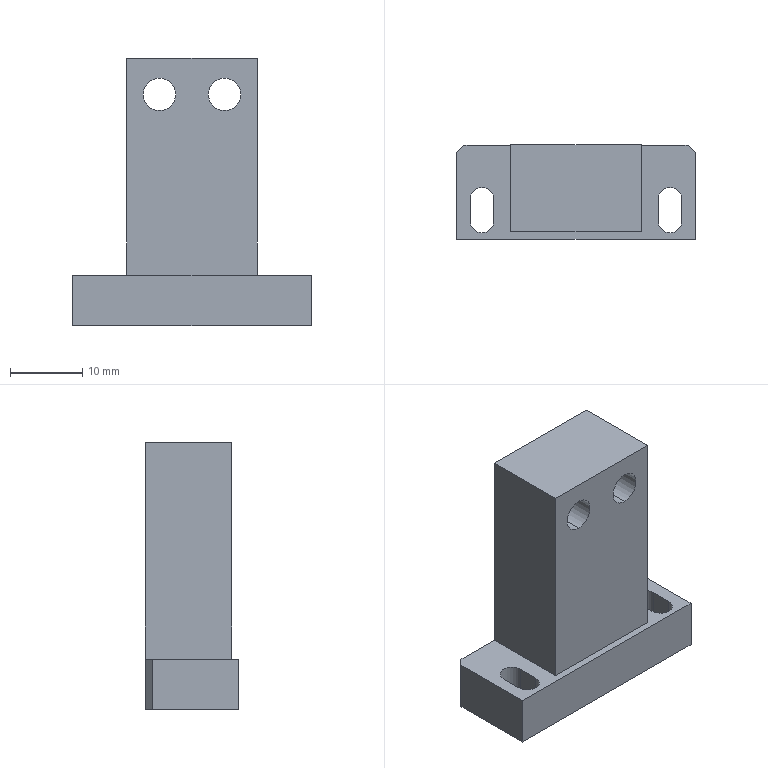Part | NX | features BREP 1 | 1 solid | 34 faces | box 33 x 13 x 37 mm | volume 8386 mm3 | plane 18 | cylinder 14 | cone 2 | commonest cylinder face diameters 3.3 x4 4.5 x4 8 x4 2.5 x2
STEP:
#1=CARTESIAN_POINT('',(0.,6.5,23.75));
#2=VERTEX_POINT('',#1);
#3=CARTESIAN_POINT('',(0.,-1.,23.75));
#4=VERTEX_POINT('',#3);
#5=CARTESIAN_POINT('',(0.,6.5,23.75));
#6=DIRECTION('',(0.,1.,0.));
#7=VECTOR('',#6,1000.);
#8=LINE('',#5,#7);
#9=EDGE_CURVE('',#2,#4,#8,.F.);
#10=ORIENTED_EDGE('',*,*,#9,.T.);
#11=CARTESIAN_POINT('',(0.,-1.,26.25));
#12=VERTEX_POINT('',#11);
#13=CARTESIAN_POINT('',(0.,-1.,25.));
#14=DIRECTION('',(0.,1.,0.));
#15=DIRECTION('',(0.,0.,1.));
#16=AXIS2_PLACEMENT_3D('',#13,#14,#15);
#17=CIRCLE('',#16,1.25);
#18=EDGE_CURVE('',#12,#4,#17,.T.);
#19=ORIENTED_EDGE('',*,*,#18,.F.);
#20=CARTESIAN_POINT('',(0.,6.5,26.25));
#21=VERTEX_POINT('',#20);
#22=CARTESIAN_POINT('',(0.,6.5,26.25));
#23=DIRECTION('',(0.,1.,0.));
#24=VECTOR('',#23,1000.);
#25=LINE('',#22,#24);
#26=EDGE_CURVE('',#21,#12,#25,.F.);
#27=ORIENTED_EDGE('',*,*,#26,.F.);
#28=CARTESIAN_POINT('',(0.,6.5,25.));
#29=DIRECTION('',(0.,1.,0.));
#30=DIRECTION('',(0.,0.,1.));
#31=AXIS2_PLACEMENT_3D('',#28,#29,#30);
#32=CIRCLE('',#31,1.25);
#33=EDGE_CURVE('',#21,#2,#32,.T.);
#34=ORIENTED_EDGE('',*,*,#33,.T.);
#35=EDGE_LOOP('',(#10,#19,#27,#34));
#36=FACE_BOUND('',#35,.T.);
#37=CARTESIAN_POINT('',(0.,6.5,25.));
#38=DIRECTION('',(0.,1.,0.));
#39=DIRECTION('',(0.,0.,1.));
#40=AXIS2_PLACEMENT_3D('',#37,#38,#39);
#41=CYLINDRICAL_SURFACE('',#40,1.25);
#42=ADVANCED_FACE('',(#36),#41,.F.);
#43=CARTESIAN_POINT('',(0.,-1.751,25.));
#44=VERTEX_POINT('',#43);
#45=CARTESIAN_POINT('',(0.,-1.,23.75));
#46=DIRECTION('',(0.,0.515,-0.8572));
#47=VECTOR('',#46,1000.);
#48=LINE('',#45,#47);
#49=EDGE_CURVE('',#44,#4,#48,.T.);
#50=ORIENTED_EDGE('',*,*,#49,.F.);
#51=CARTESIAN_POINT('',(0.,-1.,26.25));
#52=DIRECTION('',(0.,0.515,0.8572));
#53=VECTOR('',#52,1000.);
#54=LINE('',#51,#53);
#55=EDGE_CURVE('',#44,#12,#54,.T.);
#56=ORIENTED_EDGE('',*,*,#55,.T.);
#57=ORIENTED_EDGE('',*,*,#18,.T.);
#58=EDGE_LOOP('',(#50,#56,#57));
#59=FACE_BOUND('',#58,.T.);
#60=CARTESIAN_POINT('',(0.,-1.,25.));
#61=DIRECTION('',(0.,1.,0.));
#62=DIRECTION('',(0.,0.,1.));
#63=AXIS2_PLACEMENT_3D('',#60,#61,#62);
#64=CONICAL_SURFACE('',#63,1.25,1.03);
#65=ADVANCED_FACE('',(#59),#64,.F.);
#66=CARTESIAN_POINT('',(4.5,6.5,28.));
#67=VERTEX_POINT('',#66);
#68=CARTESIAN_POINT('',(4.5,0.5,28.));
#69=VERTEX_POINT('',#68);
#70=CARTESIAN_POINT('',(4.5,6.5,28.));
#71=DIRECTION('',(0.,1.,0.));
#72=VECTOR('',#71,1000.);
#73=LINE('',#70,#72);
#74=EDGE_CURVE('',#67,#69,#73,.F.);
#75=ORIENTED_EDGE('',*,*,#74,.T.);
#76=CARTESIAN_POINT('',(4.5,0.5,36.));
#77=VERTEX_POINT('',#76);
#78=CARTESIAN_POINT('',(4.5,0.5,32.));
#79=DIRECTION('',(0.,1.,0.));
#80=DIRECTION('',(0.,0.,1.));
#81=AXIS2_PLACEMENT_3D('',#78,#79,#80);
#82=CIRCLE('',#81,4.);
#83=EDGE_CURVE('',#77,#69,#82,.T.);
#84=ORIENTED_EDGE('',*,*,#83,.F.);
#85=CARTESIAN_POINT('',(4.5,6.5,36.));
#86=VERTEX_POINT('',#85);
#87=CARTESIAN_POINT('',(4.5,6.5,36.));
#88=DIRECTION('',(0.,1.,0.));
#89=VECTOR('',#88,1000.);
#90=LINE('',#87,#89);
#91=EDGE_CURVE('',#86,#77,#90,.F.);
#92=ORIENTED_EDGE('',*,*,#91,.F.);
#93=CARTESIAN_POINT('',(4.5,6.5,32.));
#94=DIRECTION('',(0.,1.,0.));
#95=DIRECTION('',(0.,0.,1.));
#96=AXIS2_PLACEMENT_3D('',#93,#94,#95);
#97=CIRCLE('',#96,4.);
#98=EDGE_CURVE('',#86,#67,#97,.T.);
#99=ORIENTED_EDGE('',*,*,#98,.T.);
#100=EDGE_LOOP('',(#75,#84,#92,#99));
#101=FACE_BOUND('',#100,.T.);
#102=CARTESIAN_POINT('',(4.5,6.5,32.));
#103=DIRECTION('',(0.,1.,0.));
#104=DIRECTION('',(0.,0.,1.));
#105=AXIS2_PLACEMENT_3D('',#102,#103,#104);
#106=CYLINDRICAL_SURFACE('',#105,4.);
#107=ADVANCED_FACE('',(#101),#106,.F.);
#108=ORIENTED_EDGE('',*,*,#83,.T.);
#109=CARTESIAN_POINT('',(4.5,0.5,32.));
#110=DIRECTION('',(0.,1.,0.));
#111=DIRECTION('',(0.,0.,1.));
#112=AXIS2_PLACEMENT_3D('',#109,#110,#111);
#113=CIRCLE('',#112,4.);
#114=EDGE_CURVE('',#69,#77,#113,.T.);
#115=ORIENTED_EDGE('',*,*,#114,.T.);
#116=EDGE_LOOP('',(#108,#115));
#117=FACE_BOUND('',#116,.T.);
#118=CARTESIAN_POINT('',(4.5,0.5,34.25));
#119=VERTEX_POINT('',#118);
#120=CARTESIAN_POINT('',(4.5,0.5,29.75));
#121=VERTEX_POINT('',#120);
#122=CARTESIAN_POINT('',(4.5,0.5,32.));
#123=DIRECTION('',(0.,1.,0.));
#124=DIRECTION('',(0.,0.,1.));
#125=AXIS2_PLACEMENT_3D('',#122,#123,#124);
#126=CIRCLE('',#125,2.25);
#127=EDGE_CURVE('',#119,#121,#126,.T.);
#128=ORIENTED_EDGE('',*,*,#127,.F.);
#129=CARTESIAN_POINT('',(4.5,0.5,32.));
#130=DIRECTION('',(0.,1.,0.));
#131=DIRECTION('',(0.,0.,1.));
#132=AXIS2_PLACEMENT_3D('',#129,#130,#131);
#133=CIRCLE('',#132,2.25);
#134=EDGE_CURVE('',#121,#119,#133,.T.);
#135=ORIENTED_EDGE('',*,*,#134,.F.);
#136=EDGE_LOOP('',(#128,#135));
#137=FACE_BOUND('',#136,.T.);
#138=CARTESIAN_POINT('',(6.75,0.5,32.));
#139=DIRECTION('',(0.,-1.,0.));
#140=DIRECTION('',(0.,0.,-1.));
#141=AXIS2_PLACEMENT_3D('',#138,#139,#140);
#142=PLANE('',#141);
#143=ADVANCED_FACE('',(#117,#137),#142,.F.);
#144=CARTESIAN_POINT('',(4.5,-5.5,29.75));
#145=VERTEX_POINT('',#144);
#146=CARTESIAN_POINT('',(4.5,6.5,29.75));
#147=DIRECTION('',(0.,1.,0.));
#148=VECTOR('',#147,1000.);
#149=LINE('',#146,#148);
#150=EDGE_CURVE('',#121,#145,#149,.F.);
#151=ORIENTED_EDGE('',*,*,#150,.T.);
#152=CARTESIAN_POINT('',(4.5,-5.5,34.25));
#153=VERTEX_POINT('',#152);
#154=CARTESIAN_POINT('',(4.5,-5.5,32.));
#155=DIRECTION('',(0.,1.,0.));
#156=DIRECTION('',(-1.,0.,0.));
#157=AXIS2_PLACEMENT_3D('',#154,#155,#156);
#158=CIRCLE('',#157,2.25);
#159=EDGE_CURVE('',#153,#145,#158,.T.);
#160=ORIENTED_EDGE('',*,*,#159,.F.);
#161=CARTESIAN_POINT('',(4.5,6.5,34.25));
#162=DIRECTION('',(0.,1.,0.));
#163=VECTOR('',#162,1000.);
#164=LINE('',#161,#163);
#165=EDGE_CURVE('',#119,#153,#164,.F.);
#166=ORIENTED_EDGE('',*,*,#165,.F.);
#167=ORIENTED_EDGE('',*,*,#127,.T.);
#168=EDGE_LOOP('',(#151,#160,#166,#167));
#169=FACE_BOUND('',#168,.T.);
#170=CARTESIAN_POINT('',(4.5,6.5,32.));
#171=DIRECTION('',(0.,1.,0.));
#172=DIRECTION('',(0.,0.,1.));
#173=AXIS2_PLACEMENT_3D('',#170,#171,#172);
#174=CYLINDRICAL_SURFACE('',#173,2.25);
#175=ADVANCED_FACE('',(#169),#174,.F.);
#176=CARTESIAN_POINT('',(-4.5,6.5,28.));
#177=VERTEX_POINT('',#176);
#178=CARTESIAN_POINT('',(-4.5,0.5,28.));
#179=VERTEX_POINT('',#178);
#180=CARTESIAN_POINT('',(-4.5,6.5,28.));
#181=DIRECTION('',(0.,1.,0.));
#182=VECTOR('',#181,1000.);
#183=LINE('',#180,#182);
#184=EDGE_CURVE('',#177,#179,#183,.F.);
#185=ORIENTED_EDGE('',*,*,#184,.T.);
#186=CARTESIAN_POINT('',(-4.5,0.5,36.));
#187=VERTEX_POINT('',#186);
#188=CARTESIAN_POINT('',(-4.5,0.5,32.));
#189=DIRECTION('',(0.,1.,0.));
#190=DIRECTION('',(0.,0.,1.));
#191=AXIS2_PLACEMENT_3D('',#188,#189,#190);
#192=CIRCLE('',#191,4.);
#193=EDGE_CURVE('',#187,#179,#192,.T.);
#194=ORIENTED_EDGE('',*,*,#193,.F.);
#195=CARTESIAN_POINT('',(-4.5,6.5,36.));
#196=VERTEX_POINT('',#195);
#197=CARTESIAN_POINT('',(-4.5,6.5,36.));
#198=DIRECTION('',(0.,1.,0.));
#199=VECTOR('',#198,1000.);
#200=LINE('',#197,#199);
#201=EDGE_CURVE('',#196,#187,#200,.F.);
#202=ORIENTED_EDGE('',*,*,#201,.F.);
#203=CARTESIAN_POINT('',(-4.5,6.5,32.));
#204=DIRECTION('',(0.,1.,0.));
#205=DIRECTION('',(0.,0.,1.));
#206=AXIS2_PLACEMENT_3D('',#203,#204,#205);
#207=CIRCLE('',#206,4.);
#208=EDGE_CURVE('',#196,#177,#207,.T.);
#209=ORIENTED_EDGE('',*,*,#208,.T.);
#210=EDGE_LOOP('',(#185,#194,#202,#209));
#211=FACE_BOUND('',#210,.T.);
#212=CARTESIAN_POINT('',(-4.5,6.5,32.));
#213=DIRECTION('',(0.,1.,0.));
#214=DIRECTION('',(0.,0.,1.));
#215=AXIS2_PLACEMENT_3D('',#212,#213,#214);
#216=CYLINDRICAL_SURFACE('',#215,4.);
#217=ADVANCED_FACE('',(#211),#216,.F.);
#218=ORIENTED_EDGE('',*,*,#193,.T.);
#219=CARTESIAN_POINT('',(-4.5,0.5,32.));
#220=DIRECTION('',(0.,1.,0.));
#221=DIRECTION('',(0.,0.,1.));
#222=AXIS2_PLACEMENT_3D('',#219,#220,#221);
#223=CIRCLE('',#222,4.);
#224=EDGE_CURVE('',#179,#187,#223,.T.);
#225=ORIENTED_EDGE('',*,*,#224,.T.);
#226=EDGE_LOOP('',(#218,#225));
#227=FACE_BOUND('',#226,.T.);
#228=CARTESIAN_POINT('',(-4.5,0.5,34.25));
#229=VERTEX_POINT('',#228);
#230=CARTESIAN_POINT('',(-4.5,0.5,29.75));
#231=VERTEX_POINT('',#230);
#232=CARTESIAN_POINT('',(-4.5,0.5,32.));
#233=DIRECTION('',(0.,1.,0.));
#234=DIRECTION('',(0.,0.,1.));
#235=AXIS2_PLACEMENT_3D('',#232,#233,#234);
#236=CIRCLE('',#235,2.25);
#237=EDGE_CURVE('',#229,#231,#236,.T.);
#238=ORIENTED_EDGE('',*,*,#237,.F.);
#239=CARTESIAN_POINT('',(-4.5,0.5,32.));
#240=DIRECTION('',(0.,1.,0.));
#241=DIRECTION('',(0.,0.,1.));
#242=AXIS2_PLACEMENT_3D('',#239,#240,#241);
#243=CIRCLE('',#242,2.25);
#244=EDGE_CURVE('',#231,#229,#243,.T.);
#245=ORIENTED_EDGE('',*,*,#244,.F.);
#246=EDGE_LOOP('',(#238,#245));
#247=FACE_BOUND('',#246,.T.);
#248=CARTESIAN_POINT('',(-2.25,0.5,32.));
#249=DIRECTION('',(0.,-1.,0.));
#250=DIRECTION('',(0.,0.,-1.));
#251=AXIS2_PLACEMENT_3D('',#248,#249,#250);
#252=PLANE('',#251);
#253=ADVANCED_FACE('',(#227,#247),#252,.F.);
#254=CARTESIAN_POINT('',(-4.5,-5.5,29.75));
#255=VERTEX_POINT('',#254);
#256=CARTESIAN_POINT('',(-4.5,6.5,29.75));
#257=DIRECTION('',(0.,1.,0.));
#258=VECTOR('',#257,1000.);
#259=LINE('',#256,#258);
#260=EDGE_CURVE('',#231,#255,#259,.F.);
#261=ORIENTED_EDGE('',*,*,#260,.T.);
#262=CARTESIAN_POINT('',(-4.5,-5.5,34.25));
#263=VERTEX_POINT('',#262);
#264=CARTESIAN_POINT('',(-4.5,-5.5,32.));
#265=DIRECTION('',(0.,1.,0.));
#266=DIRECTION('',(-1.,0.,0.));
#267=AXIS2_PLACEMENT_3D('',#264,#265,#266);
#268=CIRCLE('',#267,2.25);
#269=EDGE_CURVE('',#263,#255,#268,.T.);
#270=ORIENTED_EDGE('',*,*,#269,.F.);
#271=CARTESIAN_POINT('',(-4.5,6.5,34.25));
#272=DIRECTION('',(0.,1.,0.));
#273=VECTOR('',#272,1000.);
#274=LINE('',#271,#273);
#275=EDGE_CURVE('',#229,#263,#274,.F.);
#276=ORIENTED_EDGE('',*,*,#275,.F.);
#277=ORIENTED_EDGE('',*,*,#237,.T.);
#278=EDGE_LOOP('',(#261,#270,#276,#277));
#279=FACE_BOUND('',#278,.T.);
#280=CARTESIAN_POINT('',(-4.5,6.5,32.));
#281=DIRECTION('',(0.,1.,0.));
#282=DIRECTION('',(0.,0.,1.));
#283=AXIS2_PLACEMENT_3D('',#280,#281,#282);
#284=CYLINDRICAL_SURFACE('',#283,2.25);
#285=ADVANCED_FACE('',(#279),#284,.F.);
#286=CARTESIAN_POINT('',(-15.5,6.5,7.));
#287=VERTEX_POINT('',#286);
#288=CARTESIAN_POINT('',(-16.5,5.5,7.));
#289=VERTEX_POINT('',#288);
#290=CARTESIAN_POINT('',(-11.,11.,7.));
#291=DIRECTION('',(-0.7071,-0.7071,0.));
#292=VECTOR('',#291,1000.);
#293=LINE('',#290,#292);
#294=EDGE_CURVE('',#287,#289,#293,.T.);
#295=ORIENTED_EDGE('',*,*,#294,.F.);
#296=CARTESIAN_POINT('',(-15.5,6.5,0.));
#297=VERTEX_POINT('',#296);
#298=CARTESIAN_POINT('',(-15.5,6.5,7.));
#299=DIRECTION('',(0.,0.,1.));
#300=VECTOR('',#299,1000.);
#301=LINE('',#298,#300);
#302=EDGE_CURVE('',#297,#287,#301,.T.);
#303=ORIENTED_EDGE('',*,*,#302,.F.);
#304=CARTESIAN_POINT('',(-16.5,5.5,0.));
#305=VERTEX_POINT('',#304);
#306=CARTESIAN_POINT('',(-16.5,5.5,0.));
#307=DIRECTION('',(0.7071,0.7071,0.));
#308=VECTOR('',#307,1000.);
#309=LINE('',#306,#308);
#310=EDGE_CURVE('',#305,#297,#309,.T.);
#311=ORIENTED_EDGE('',*,*,#310,.F.);
#312=CARTESIAN_POINT('',(-16.5,5.5,7.));
#313=DIRECTION('',(0.,0.,-1.));
#314=VECTOR('',#313,1000.);
#315=LINE('',#312,#314);
#316=EDGE_CURVE('',#289,#305,#315,.T.);
#317=ORIENTED_EDGE('',*,*,#316,.F.);
#318=EDGE_LOOP('',(#295,#303,#311,#317));
#319=FACE_BOUND('',#318,.T.);
#320=CARTESIAN_POINT('',(-16.5,5.5,7.));
#321=DIRECTION('',(0.7071,-0.7071,0.));
#322=DIRECTION('',(0.,0.,-1.));
#323=AXIS2_PLACEMENT_3D('',#320,#321,#322);
#324=PLANE('',#323);
#325=ADVANCED_FACE('',(#319),#324,.F.);
#326=CARTESIAN_POINT('',(16.5,5.5,7.));
#327=VERTEX_POINT('',#326);
#328=CARTESIAN_POINT('',(15.5,6.5,7.));
#329=VERTEX_POINT('',#328);
#330=CARTESIAN_POINT('',(11.,11.,7.));
#331=DIRECTION('',(-0.7071,0.7071,0.));
#332=VECTOR('',#331,1000.);
#333=LINE('',#330,#332);
#334=EDGE_CURVE('',#327,#329,#333,.T.);
#335=ORIENTED_EDGE('',*,*,#334,.F.);
#336=CARTESIAN_POINT('',(16.5,5.5,0.));
#337=VERTEX_POINT('',#336);
#338=CARTESIAN_POINT('',(16.5,5.5,7.));
#339=DIRECTION('',(0.,0.,1.));
#340=VECTOR('',#339,1000.);
#341=LINE('',#338,#340);
#342=EDGE_CURVE('',#337,#327,#341,.T.);
#343=ORIENTED_EDGE('',*,*,#342,.F.);
#344=CARTESIAN_POINT('',(15.5,6.5,0.));
#345=VERTEX_POINT('',#344);
#346=CARTESIAN_POINT('',(15.5,6.5,0.));
#347=DIRECTION('',(0.7071,-0.7071,0.));
#348=VECTOR('',#347,1000.);
#349=LINE('',#346,#348);
#350=EDGE_CURVE('',#345,#337,#349,.T.);
#351=ORIENTED_EDGE('',*,*,#350,.F.);
#352=CARTESIAN_POINT('',(15.5,6.5,7.));
#353=DIRECTION('',(0.,0.,-1.));
#354=VECTOR('',#353,1000.);
#355=LINE('',#352,#354);
#356=EDGE_CURVE('',#329,#345,#355,.T.);
#357=ORIENTED_EDGE('',*,*,#356,.F.);
#358=EDGE_LOOP('',(#335,#343,#351,#357));
#359=FACE_BOUND('',#358,.T.);
#360=CARTESIAN_POINT('',(15.5,6.5,7.));
#361=DIRECTION('',(-0.7071,-0.7071,0.));
#362=DIRECTION('',(0.,0.,-1.));
#363=AXIS2_PLACEMENT_3D('',#360,#361,#362);
#364=PLANE('',#363);
#365=ADVANCED_FACE('',(#359),#364,.F.);
#366=CARTESIAN_POINT('',(-14.65,-4.,0.));
#367=VERTEX_POINT('',#366);
#368=CARTESIAN_POINT('',(-14.65,-1.,0.));
#369=VERTEX_POINT('',#368);
#370=CARTESIAN_POINT('',(-14.65,-1.,0.));
#371=DIRECTION('',(0.,1.,0.));
#372=VECTOR('',#371,1000.);
#373=LINE('',#370,#372);
#374=EDGE_CURVE('',#367,#369,#373,.T.);
#375=ORIENTED_EDGE('',*,*,#374,.T.);
#376=CARTESIAN_POINT('',(-14.65,-1.,7.));
#377=VERTEX_POINT('',#376);
#378=CARTESIAN_POINT('',(-14.65,-1.,-0.001));
#379=DIRECTION('',(0.,0.,1.));
#380=VECTOR('',#379,1000.);
#381=LINE('',#378,#380);
#382=EDGE_CURVE('',#369,#377,#381,.T.);
#383=ORIENTED_EDGE('',*,*,#382,.T.);
#384=CARTESIAN_POINT('',(-14.65,-4.,7.));
#385=VERTEX_POINT('',#384);
#386=CARTESIAN_POINT('',(-14.65,-1.,7.));
#387=DIRECTION('',(0.,-1.,0.));
#388=VECTOR('',#387,1000.);
#389=LINE('',#386,#388);
#390=EDGE_CURVE('',#377,#385,#389,.T.);
#391=ORIENTED_EDGE('',*,*,#390,.T.);
#392=CARTESIAN_POINT('',(-14.65,-4.,-0.001));
#393=DIRECTION('',(0.,0.,1.));
#394=VECTOR('',#393,1000.);
#395=LINE('',#392,#394);
#396=EDGE_CURVE('',#367,#385,#395,.T.);
#397=ORIENTED_EDGE('',*,*,#396,.F.);
#398=EDGE_LOOP('',(#375,#383,#391,#397));
#399=FACE_BOUND('',#398,.T.);
#400=CARTESIAN_POINT('',(-14.65,-1.,-0.001));
#401=DIRECTION('',(-1.,0.,0.));
#402=DIRECTION('',(0.,0.,1.));
#403=AXIS2_PLACEMENT_3D('',#400,#401,#402);
#404=PLANE('',#403);
#405=ADVANCED_FACE('',(#399),#404,.F.);
#406=CARTESIAN_POINT('',(-11.35,-4.,0.));
#407=VERTEX_POINT('',#406);
#408=CARTESIAN_POINT('',(-13.,-4.,0.));
#409=DIRECTION('',(0.,0.,-1.));
#410=DIRECTION('',(1.,0.,0.));
#411=AXIS2_PLACEMENT_3D('',#408,#409,#410);
#412=CIRCLE('',#411,1.65);
#413=EDGE_CURVE('',#407,#367,#412,.T.);
#414=ORIENTED_EDGE('',*,*,#413,.T.);
#415=ORIENTED_EDGE('',*,*,#396,.T.);
#416=CARTESIAN_POINT('',(-11.35,-4.,7.));
#417=VERTEX_POINT('',#416);
#418=CARTESIAN_POINT('',(-13.,-4.,7.));
#419=DIRECTION('',(0.,0.,1.));
#420=DIRECTION('',(-1.,0.,0.));
#421=AXIS2_PLACEMENT_3D('',#418,#419,#420);
#422=CIRCLE('',#421,1.65);
#423=EDGE_CURVE('',#385,#417,#422,.T.);
#424=ORIENTED_EDGE('',*,*,#423,.T.);
#425=CARTESIAN_POINT('',(-11.35,-4.,-0.001));
#426=DIRECTION('',(0.,0.,1.));
#427=VECTOR('',#426,1000.);
#428=LINE('',#425,#427);
#429=EDGE_CURVE('',#407,#417,#428,.T.);
#430=ORIENTED_EDGE('',*,*,#429,.F.);
#431=EDGE_LOOP('',(#414,#415,#424,#430));
#432=FACE_BOUND('',#431,.T.);
#433=CARTESIAN_POINT('',(-13.,-4.,-0.001));
#434=DIRECTION('',(0.,0.,1.));
#435=DIRECTION('',(1.,0.,0.));
#436=AXIS2_PLACEMENT_3D('',#433,#434,#435);
#437=CYLINDRICAL_SURFACE('',#436,1.65);
#438=ADVANCED_FACE('',(#432),#437,.F.);
#439=CARTESIAN_POINT('',(-11.35,-1.,0.));
#440=VERTEX_POINT('',#439);
#441=CARTESIAN_POINT('',(-11.35,-1.,0.));
#442=DIRECTION('',(0.,-1.,0.));
#443=VECTOR('',#442,1000.);
#444=LINE('',#441,#443);
#445=EDGE_CURVE('',#440,#407,#444,.T.);
#446=ORIENTED_EDGE('',*,*,#445,.T.);
#447=ORIENTED_EDGE('',*,*,#429,.T.);
#448=CARTESIAN_POINT('',(-11.35,-1.,7.));
#449=VERTEX_POINT('',#448);
#450=CARTESIAN_POINT('',(-11.35,-1.,7.));
#451=DIRECTION('',(0.,1.,0.));
#452=VECTOR('',#451,1000.);
#453=LINE('',#450,#452);
#454=EDGE_CURVE('',#417,#449,#453,.T.);
#455=ORIENTED_EDGE('',*,*,#454,.T.);
#456=CARTESIAN_POINT('',(-11.35,-1.,-0.001));
#457=DIRECTION('',(0.,0.,1.));
#458=VECTOR('',#457,1000.);
#459=LINE('',#456,#458);
#460=EDGE_CURVE('',#440,#449,#459,.T.);
#461=ORIENTED_EDGE('',*,*,#460,.F.);
#462=EDGE_LOOP('',(#446,#447,#455,#461));
#463=FACE_BOUND('',#462,.T.);
#464=CARTESIAN_POINT('',(-11.35,-1.,-0.001));
#465=DIRECTION('',(1.,0.,0.));
#466=DIRECTION('',(0.,0.,-1.));
#467=AXIS2_PLACEMENT_3D('',#464,#465,#466);
#468=PLANE('',#467);
#469=ADVANCED_FACE('',(#463),#468,.F.);
#470=CARTESIAN_POINT('',(-13.,-1.,0.));
#471=DIRECTION('',(0.,0.,-1.));
#472=DIRECTION('',(1.,0.,0.));
#473=AXIS2_PLACEMENT_3D('',#470,#471,#472);
#474=CIRCLE('',#473,1.65);
#475=EDGE_CURVE('',#369,#440,#474,.T.);
#476=ORIENTED_EDGE('',*,*,#475,.T.);
#477=ORIENTED_EDGE('',*,*,#460,.T.);
#478=CARTESIAN_POINT('',(-13.,-1.,7.));
#479=DIRECTION('',(0.,0.,1.));
#480=DIRECTION('',(-1.,0.,0.));
#481=AXIS2_PLACEMENT_3D('',#478,#479,#480);
#482=CIRCLE('',#481,1.65);
#483=EDGE_CURVE('',#449,#377,#482,.T.);
#484=ORIENTED_EDGE('',*,*,#483,.T.);
#485=ORIENTED_EDGE('',*,*,#382,.F.);
#486=EDGE_LOOP('',(#476,#477,#484,#485));
#487=FACE_BOUND('',#486,.T.);
#488=CARTESIAN_POINT('',(-13.,-1.,-0.001));
#489=DIRECTION('',(0.,0.,1.));
#490=DIRECTION('',(1.,0.,0.));
#491=AXIS2_PLACEMENT_3D('',#488,#489,#490);
#492=CYLINDRICAL_SURFACE('',#491,1.65);
#493=ADVANCED_FACE('',(#487),#492,.F.);
#494=CARTESIAN_POINT('',(11.35,-4.,0.));
#495=VERTEX_POINT('',#494);
#496=CARTESIAN_POINT('',(11.35,-1.,0.));
#497=VERTEX_POINT('',#496);
#498=CARTESIAN_POINT('',(11.35,-1.,0.));
#499=DIRECTION('',(0.,1.,0.));
#500=VECTOR('',#499,1000.);
#501=LINE('',#498,#500);
#502=EDGE_CURVE('',#495,#497,#501,.T.);
#503=ORIENTED_EDGE('',*,*,#502,.T.);
#504=CARTESIAN_POINT('',(11.35,-1.,7.));
#505=VERTEX_POINT('',#504);
#506=CARTESIAN_POINT('',(11.35,-1.,-0.001));
#507=DIRECTION('',(0.,0.,1.));
#508=VECTOR('',#507,1000.);
#509=LINE('',#506,#508);
#510=EDGE_CURVE('',#497,#505,#509,.T.);
#511=ORIENTED_EDGE('',*,*,#510,.T.);
#512=CARTESIAN_POINT('',(11.35,-4.,7.));
#513=VERTEX_POINT('',#512);
#514=CARTESIAN_POINT('',(11.35,-1.,7.));
#515=DIRECTION('',(0.,-1.,0.));
#516=VECTOR('',#515,1000.);
#517=LINE('',#514,#516);
#518=EDGE_CURVE('',#505,#513,#517,.T.);
#519=ORIENTED_EDGE('',*,*,#518,.T.);
#520=CARTESIAN_POINT('',(11.35,-4.,-0.001));
#521=DIRECTION('',(0.,0.,1.));
#522=VECTOR('',#521,1000.);
#523=LINE('',#520,#522);
#524=EDGE_CURVE('',#495,#513,#523,.T.);
#525=ORIENTED_EDGE('',*,*,#524,.F.);
#526=EDGE_LOOP('',(#503,#511,#519,#525));
#527=FACE_BOUND('',#526,.T.);
#528=CARTESIAN_POINT('',(11.35,-1.,-0.001));
#529=DIRECTION('',(-1.,0.,0.));
#530=DIRECTION('',(0.,0.,1.));
#531=AXIS2_PLACEMENT_3D('',#528,#529,#530);
#532=PLANE('',#531);
#533=ADVANCED_FACE('',(#527),#532,.F.);
#534=CARTESIAN_POINT('',(14.65,-4.,0.));
#535=VERTEX_POINT('',#534);
#536=CARTESIAN_POINT('',(13.,-4.,0.));
#537=DIRECTION('',(0.,0.,-1.));
#538=DIRECTION('',(1.,0.,0.));
#539=AXIS2_PLACEMENT_3D('',#536,#537,#538);
#540=CIRCLE('',#539,1.65);
#541=EDGE_CURVE('',#535,#495,#540,.T.);
#542=ORIENTED_EDGE('',*,*,#541,.T.);
#543=ORIENTED_EDGE('',*,*,#524,.T.);
#544=CARTESIAN_POINT('',(14.65,-4.,7.));
#545=VERTEX_POINT('',#544);
#546=CARTESIAN_POINT('',(13.,-4.,7.));
#547=DIRECTION('',(0.,0.,1.));
#548=DIRECTION('',(1.,0.,0.));
#549=AXIS2_PLACEMENT_3D('',#546,#547,#548);
#550=CIRCLE('',#549,1.65);
#551=EDGE_CURVE('',#513,#545,#550,.T.);
#552=ORIENTED_EDGE('',*,*,#551,.T.);
#553=CARTESIAN_POINT('',(14.65,-4.,-0.001));
#554=DIRECTION('',(0.,0.,1.));
#555=VECTOR('',#554,1000.);
#556=LINE('',#553,#555);
#557=EDGE_CURVE('',#535,#545,#556,.T.);
#558=ORIENTED_EDGE('',*,*,#557,.F.);
#559=EDGE_LOOP('',(#542,#543,#552,#558));
#560=FACE_BOUND('',#559,.T.);
#561=CARTESIAN_POINT('',(13.,-4.,-0.001));
#562=DIRECTION('',(0.,0.,1.));
#563=DIRECTION('',(1.,0.,0.));
#564=AXIS2_PLACEMENT_3D('',#561,#562,#563);
#565=CYLINDRICAL_SURFACE('',#564,1.65);
#566=ADVANCED_FACE('',(#560),#565,.F.);
#567=CARTESIAN_POINT('',(14.65,-1.,0.));
#568=VERTEX_POINT('',#567);
#569=CARTESIAN_POINT('',(14.65,-1.,0.));
#570=DIRECTION('',(0.,-1.,0.));
#571=VECTOR('',#570,1000.);
#572=LINE('',#569,#571);
#573=EDGE_CURVE('',#568,#535,#572,.T.);
#574=ORIENTED_EDGE('',*,*,#573,.T.);
#575=ORIENTED_EDGE('',*,*,#557,.T.);
#576=CARTESIAN_POINT('',(14.65,-1.,7.));
#577=VERTEX_POINT('',#576);
#578=CARTESIAN_POINT('',(14.65,-1.,7.));
#579=DIRECTION('',(0.,1.,0.));
#580=VECTOR('',#579,1000.);
#581=LINE('',#578,#580);
#582=EDGE_CURVE('',#545,#577,#581,.T.);
#583=ORIENTED_EDGE('',*,*,#582,.T.);
#584=CARTESIAN_POINT('',(14.65,-1.,-0.001));
#585=DIRECTION('',(0.,0.,1.));
#586=VECTOR('',#585,1000.);
#587=LINE('',#584,#586);
#588=EDGE_CURVE('',#568,#577,#587,.T.);
#589=ORIENTED_EDGE('',*,*,#588,.F.);
#590=EDGE_LOOP('',(#574,#575,#583,#589));
#591=FACE_BOUND('',#590,.T.);
#592=CARTESIAN_POINT('',(14.65,-1.,-0.001));
#593=DIRECTION('',(1.,0.,0.));
#594=DIRECTION('',(0.,0.,-1.));
#595=AXIS2_PLACEMENT_3D('',#592,#593,#594);
#596=PLANE('',#595);
#597=ADVANCED_FACE('',(#591),#596,.F.);
#598=CARTESIAN_POINT('',(13.,-1.,0.));
#599=DIRECTION('',(0.,0.,-1.));
#600=DIRECTION('',(1.,0.,0.));
#601=AXIS2_PLACEMENT_3D('',#598,#599,#600);
#602=CIRCLE('',#601,1.65);
#603=EDGE_CURVE('',#497,#568,#602,.T.);
#604=ORIENTED_EDGE('',*,*,#603,.T.);
#605=ORIENTED_EDGE('',*,*,#588,.T.);
#606=CARTESIAN_POINT('',(13.,-1.,7.));
#607=DIRECTION('',(0.,0.,1.));
#608=DIRECTION('',(1.,0.,0.));
#609=AXIS2_PLACEMENT_3D('',#606,#607,#608);
#610=CIRCLE('',#609,1.65);
#611=EDGE_CURVE('',#577,#505,#610,.T.);
#612=ORIENTED_EDGE('',*,*,#611,.T.);
#613=ORIENTED_EDGE('',*,*,#510,.F.);
#614=EDGE_LOOP('',(#604,#605,#612,#613));
#615=FACE_BOUND('',#614,.T.);
#616=CARTESIAN_POINT('',(13.,-1.,-0.001));
#617=DIRECTION('',(0.,0.,1.));
#618=DIRECTION('',(1.,0.,0.));
#619=AXIS2_PLACEMENT_3D('',#616,#617,#618);
#620=CYLINDRICAL_SURFACE('',#619,1.65);
#621=ADVANCED_FACE('',(#615),#620,.F.);
#622=CARTESIAN_POINT('',(-9.,6.5,37.));
#623=VERTEX_POINT('',#622);
#624=CARTESIAN_POINT('',(-9.,-5.5,37.));
#625=VERTEX_POINT('',#624);
#626=CARTESIAN_POINT('',(-9.,-5.5,37.));
#627=DIRECTION('',(0.,-1.,0.));
#628=VECTOR('',#627,1000.);
#629=LINE('',#626,#628);
#630=EDGE_CURVE('',#623,#625,#629,.T.);
#631=ORIENTED_EDGE('',*,*,#630,.T.);
#632=CARTESIAN_POINT('',(9.,-5.5,37.));
#633=VERTEX_POINT('',#632);
#634=CARTESIAN_POINT('',(9.,-5.5,37.));
#635=DIRECTION('',(1.,0.,0.));
#636=VECTOR('',#635,1000.);
#637=LINE('',#634,#636);
#638=EDGE_CURVE('',#625,#633,#637,.T.);
#639=ORIENTED_EDGE('',*,*,#638,.T.);
#640=CARTESIAN_POINT('',(9.,6.5,37.));
#641=VERTEX_POINT('',#640);
#642=CARTESIAN_POINT('',(9.,-5.5,37.));
#643=DIRECTION('',(0.,1.,0.));
#644=VECTOR('',#643,1000.);
#645=LINE('',#642,#644);
#646=EDGE_CURVE('',#633,#641,#645,.T.);
#647=ORIENTED_EDGE('',*,*,#646,.T.);
#648=CARTESIAN_POINT('',(9.,6.5,37.));
#649=DIRECTION('',(-1.,0.,0.));
#650=VECTOR('',#649,1000.);
#651=LINE('',#648,#650);
#652=EDGE_CURVE('',#641,#623,#651,.T.);
#653=ORIENTED_EDGE('',*,*,#652,.T.);
#654=EDGE_LOOP('',(#631,#639,#647,#653));
#655=FACE_BOUND('',#654,.T.);
#656=CARTESIAN_POINT('',(0.,0.,37.));
#657=DIRECTION('',(0.,0.,1.));
#658=DIRECTION('',(1.,0.,0.));
#659=AXIS2_PLACEMENT_3D('',#656,#657,#658);
#660=PLANE('',#659);
#661=ADVANCED_FACE('',(#655),#660,.T.);
#662=CARTESIAN_POINT('',(9.,-5.5,7.));
#663=VERTEX_POINT('',#662);
#664=CARTESIAN_POINT('',(9.,6.5,7.));
#665=VERTEX_POINT('',#664);
#666=CARTESIAN_POINT('',(9.,-5.5,7.));
#667=DIRECTION('',(0.,1.,0.));
#668=VECTOR('',#667,1000.);
#669=LINE('',#666,#668);
#670=EDGE_CURVE('',#663,#665,#669,.T.);
#671=ORIENTED_EDGE('',*,*,#670,.T.);
#672=CARTESIAN_POINT('',(9.,6.5,37.));
#673=DIRECTION('',(0.,0.,-1.));
#674=VECTOR('',#673,1000.);
#675=LINE('',#672,#674);
#676=EDGE_CURVE('',#641,#665,#675,.T.);
#677=ORIENTED_EDGE('',*,*,#676,.F.);
#678=ORIENTED_EDGE('',*,*,#646,.F.);
#679=CARTESIAN_POINT('',(9.,-5.5,37.));
#680=DIRECTION('',(0.,0.,-1.));
#681=VECTOR('',#680,1000.);
#682=LINE('',#679,#681);
#683=EDGE_CURVE('',#633,#663,#682,.T.);
#684=ORIENTED_EDGE('',*,*,#683,.T.);
#685=EDGE_LOOP('',(#671,#677,#678,#684));
#686=FACE_BOUND('',#685,.T.);
#687=CARTESIAN_POINT('',(9.,-5.5,37.));
#688=DIRECTION('',(-1.,0.,0.));
#689=DIRECTION('',(0.,0.,1.));
#690=AXIS2_PLACEMENT_3D('',#687,#688,#689);
#691=PLANE('',#690);
#692=ADVANCED_FACE('',(#686),#691,.F.);
#693=CARTESIAN_POINT('',(-9.,-5.5,7.));
#694=VERTEX_POINT('',#693);
#695=CARTESIAN_POINT('',(9.,-5.5,7.));
#696=DIRECTION('',(1.,0.,0.));
#697=VECTOR('',#696,1000.);
#698=LINE('',#695,#697);
#699=EDGE_CURVE('',#694,#663,#698,.T.);
#700=ORIENTED_EDGE('',*,*,#699,.T.);
#701=ORIENTED_EDGE('',*,*,#683,.F.);
#702=ORIENTED_EDGE('',*,*,#638,.F.);
#703=CARTESIAN_POINT('',(-9.,-5.5,37.));
#704=DIRECTION('',(0.,0.,-1.));
#705=VECTOR('',#704,1000.);
#706=LINE('',#703,#705);
#707=EDGE_CURVE('',#625,#694,#706,.T.);
#708=ORIENTED_EDGE('',*,*,#707,.T.);
#709=EDGE_LOOP('',(#700,#701,#702,#708));
#710=FACE_BOUND('',#709,.T.);
#711=ORIENTED_EDGE('',*,*,#269,.T.);
#712=CARTESIAN_POINT('',(-4.5,-5.5,32.));
#713=DIRECTION('',(0.,1.,0.));
#714=DIRECTION('',(-1.,0.,0.));
#715=AXIS2_PLACEMENT_3D('',#712,#713,#714);
#716=CIRCLE('',#715,2.25);
#717=EDGE_CURVE('',#255,#263,#716,.T.);
#718=ORIENTED_EDGE('',*,*,#717,.T.);
#719=EDGE_LOOP('',(#711,#718));
#720=FACE_BOUND('',#719,.T.);
#721=ORIENTED_EDGE('',*,*,#159,.T.);
#722=CARTESIAN_POINT('',(4.5,-5.5,32.));
#723=DIRECTION('',(0.,1.,0.));
#724=DIRECTION('',(-1.,0.,0.));
#725=AXIS2_PLACEMENT_3D('',#722,#723,#724);
#726=CIRCLE('',#725,2.25);
#727=EDGE_CURVE('',#145,#153,#726,.T.);
#728=ORIENTED_EDGE('',*,*,#727,.T.);
#729=EDGE_LOOP('',(#721,#728));
#730=FACE_BOUND('',#729,.T.);
#731=CARTESIAN_POINT('',(9.,-5.5,37.));
#732=DIRECTION('',(0.,1.,0.));
#733=DIRECTION('',(-1.,0.,0.));
#734=AXIS2_PLACEMENT_3D('',#731,#732,#733);
#735=PLANE('',#734);
#736=ADVANCED_FACE('',(#710,#720,#730),#735,.F.);
#737=CARTESIAN_POINT('',(-9.,6.5,7.));
#738=VERTEX_POINT('',#737);
#739=CARTESIAN_POINT('',(-9.,-5.5,7.));
#740=DIRECTION('',(0.,-1.,0.));
#741=VECTOR('',#740,1000.);
#742=LINE('',#739,#741);
#743=EDGE_CURVE('',#738,#694,#742,.T.);
#744=ORIENTED_EDGE('',*,*,#743,.T.);
#745=ORIENTED_EDGE('',*,*,#707,.F.);
#746=ORIENTED_EDGE('',*,*,#630,.F.);
#747=CARTESIAN_POINT('',(-9.,6.5,37.));
#748=DIRECTION('',(0.,0.,-1.));
#749=VECTOR('',#748,1000.);
#750=LINE('',#747,#749);
#751=EDGE_CURVE('',#623,#738,#750,.T.);
#752=ORIENTED_EDGE('',*,*,#751,.T.);
#753=EDGE_LOOP('',(#744,#745,#746,#752));
#754=FACE_BOUND('',#753,.T.);
#755=CARTESIAN_POINT('',(-9.,-5.5,37.));
#756=DIRECTION('',(1.,0.,0.));
#757=DIRECTION('',(0.,0.,-1.));
#758=AXIS2_PLACEMENT_3D('',#755,#756,#757);
#759=PLANE('',#758);
#760=ADVANCED_FACE('',(#754),#759,.F.);
#761=CARTESIAN_POINT('',(-16.5,6.5,0.));
#762=DIRECTION('',(-1.,0.,0.));
#763=VECTOR('',#762,1000.);
#764=LINE('',#761,#763);
#765=EDGE_CURVE('',#345,#297,#764,.T.);
#766=ORIENTED_EDGE('',*,*,#765,.F.);
#767=ORIENTED_EDGE('',*,*,#350,.T.);
#768=CARTESIAN_POINT('',(16.5,-6.5,0.));
#769=VERTEX_POINT('',#768);
#770=CARTESIAN_POINT('',(16.5,6.5,0.));
#771=DIRECTION('',(0.,1.,0.));
#772=VECTOR('',#771,1000.);
#773=LINE('',#770,#772);
#774=EDGE_CURVE('',#769,#337,#773,.T.);
#775=ORIENTED_EDGE('',*,*,#774,.F.);
#776=CARTESIAN_POINT('',(-16.5,-6.5,0.));
#777=VERTEX_POINT('',#776);
#778=CARTESIAN_POINT('',(-16.5,-6.5,0.));
#779=DIRECTION('',(1.,0.,0.));
#780=VECTOR('',#779,1000.);
#781=LINE('',#778,#780);
#782=EDGE_CURVE('',#777,#769,#781,.T.);
#783=ORIENTED_EDGE('',*,*,#782,.F.);
#784=CARTESIAN_POINT('',(-16.5,6.5,0.));
#785=DIRECTION('',(0.,-1.,0.));
#786=VECTOR('',#785,1000.);
#787=LINE('',#784,#786);
#788=EDGE_CURVE('',#305,#777,#787,.T.);
#789=ORIENTED_EDGE('',*,*,#788,.F.);
#790=ORIENTED_EDGE('',*,*,#310,.T.);
#791=EDGE_LOOP('',(#766,#767,#775,#783,#789,#790));
#792=FACE_BOUND('',#791,.T.);
#793=ORIENTED_EDGE('',*,*,#573,.F.);
#794=ORIENTED_EDGE('',*,*,#603,.F.);
#795=ORIENTED_EDGE('',*,*,#502,.F.);
#796=ORIENTED_EDGE('',*,*,#541,.F.);
#797=EDGE_LOOP('',(#793,#794,#795,#796));
#798=FACE_BOUND('',#797,.T.);
#799=ORIENTED_EDGE('',*,*,#445,.F.);
#800=ORIENTED_EDGE('',*,*,#475,.F.);
#801=ORIENTED_EDGE('',*,*,#374,.F.);
#802=ORIENTED_EDGE('',*,*,#413,.F.);
#803=EDGE_LOOP('',(#799,#800,#801,#802));
#804=FACE_BOUND('',#803,.T.);
#805=CARTESIAN_POINT('',(0.,0.,0.));
#806=DIRECTION('',(0.,0.,1.));
#807=DIRECTION('',(1.,0.,0.));
#808=AXIS2_PLACEMENT_3D('',#805,#806,#807);
#809=PLANE('',#808);
#810=ADVANCED_FACE('',(#792,#798,#804),#809,.F.);
#811=CARTESIAN_POINT('',(16.5,-6.5,7.));
#812=VERTEX_POINT('',#811);
#813=CARTESIAN_POINT('',(16.5,6.5,7.));
#814=DIRECTION('',(0.,1.,0.));
#815=VECTOR('',#814,1000.);
#816=LINE('',#813,#815);
#817=EDGE_CURVE('',#812,#327,#816,.T.);
#818=ORIENTED_EDGE('',*,*,#817,.T.);
#819=ORIENTED_EDGE('',*,*,#334,.T.);
#820=CARTESIAN_POINT('',(-16.5,6.5,7.));
#821=DIRECTION('',(-1.,0.,0.));
#822=VECTOR('',#821,1000.);
#823=LINE('',#820,#822);
#824=EDGE_CURVE('',#329,#665,#823,.T.);
#825=ORIENTED_EDGE('',*,*,#824,.T.);
#826=ORIENTED_EDGE('',*,*,#670,.F.);
#827=ORIENTED_EDGE('',*,*,#699,.F.);
#828=ORIENTED_EDGE('',*,*,#743,.F.);
#829=CARTESIAN_POINT('',(-16.5,6.5,7.));
#830=DIRECTION('',(-1.,0.,0.));
#831=VECTOR('',#830,1000.);
#832=LINE('',#829,#831);
#833=EDGE_CURVE('',#738,#287,#832,.T.);
#834=ORIENTED_EDGE('',*,*,#833,.T.);
#835=ORIENTED_EDGE('',*,*,#294,.T.);
#836=CARTESIAN_POINT('',(-16.5,-6.5,7.));
#837=VERTEX_POINT('',#836);
#838=CARTESIAN_POINT('',(-16.5,6.5,7.));
#839=DIRECTION('',(0.,-1.,0.));
#840=VECTOR('',#839,1000.);
#841=LINE('',#838,#840);
#842=EDGE_CURVE('',#289,#837,#841,.T.);
#843=ORIENTED_EDGE('',*,*,#842,.T.);
#844=CARTESIAN_POINT('',(-16.5,-6.5,7.));
#845=DIRECTION('',(1.,0.,0.));
#846=VECTOR('',#845,1000.);
#847=LINE('',#844,#846);
#848=EDGE_CURVE('',#837,#812,#847,.T.);
#849=ORIENTED_EDGE('',*,*,#848,.T.);
#850=EDGE_LOOP('',(#818,#819,#825,#826,#827,#828,#834,#835,#843,#849));
#851=FACE_BOUND('',#850,.T.);
#852=ORIENTED_EDGE('',*,*,#611,.F.);
#853=ORIENTED_EDGE('',*,*,#582,.F.);
#854=ORIENTED_EDGE('',*,*,#551,.F.);
#855=ORIENTED_EDGE('',*,*,#518,.F.);
#856=EDGE_LOOP('',(#852,#853,#854,#855));
#857=FACE_BOUND('',#856,.T.);
#858=ORIENTED_EDGE('',*,*,#483,.F.);
#859=ORIENTED_EDGE('',*,*,#454,.F.);
#860=ORIENTED_EDGE('',*,*,#423,.F.);
#861=ORIENTED_EDGE('',*,*,#390,.F.);
#862=EDGE_LOOP('',(#858,#859,#860,#861));
#863=FACE_BOUND('',#862,.T.);
#864=CARTESIAN_POINT('',(0.,0.,7.));
#865=DIRECTION('',(0.,0.,1.));
#866=DIRECTION('',(1.,0.,0.));
#867=AXIS2_PLACEMENT_3D('',#864,#865,#866);
#868=PLANE('',#867);
#869=ADVANCED_FACE('',(#851,#857,#863),#868,.T.);
#870=ORIENTED_EDGE('',*,*,#782,.T.);
#871=CARTESIAN_POINT('',(16.5,-6.5,7.));
#872=DIRECTION('',(0.,0.,-1.));
#873=VECTOR('',#872,1000.);
#874=LINE('',#871,#873);
#875=EDGE_CURVE('',#812,#769,#874,.T.);
#876=ORIENTED_EDGE('',*,*,#875,.F.);
#877=ORIENTED_EDGE('',*,*,#848,.F.);
#878=CARTESIAN_POINT('',(-16.5,-6.5,7.));
#879=DIRECTION('',(0.,0.,-1.));
#880=VECTOR('',#879,1000.);
#881=LINE('',#878,#880);
#882=EDGE_CURVE('',#837,#777,#881,.T.);
#883=ORIENTED_EDGE('',*,*,#882,.T.);
#884=EDGE_LOOP('',(#870,#876,#877,#883));
#885=FACE_BOUND('',#884,.T.);
#886=CARTESIAN_POINT('',(-16.5,-6.5,7.));
#887=DIRECTION('',(0.,1.,0.));
#888=DIRECTION('',(0.,0.,1.));
#889=AXIS2_PLACEMENT_3D('',#886,#887,#888);
#890=PLANE('',#889);
#891=ADVANCED_FACE('',(#885),#890,.F.);
#892=ORIENTED_EDGE('',*,*,#842,.F.);
#893=ORIENTED_EDGE('',*,*,#316,.T.);
#894=ORIENTED_EDGE('',*,*,#788,.T.);
#895=ORIENTED_EDGE('',*,*,#882,.F.);
#896=EDGE_LOOP('',(#892,#893,#894,#895));
#897=FACE_BOUND('',#896,.T.);
#898=CARTESIAN_POINT('',(-16.5,6.5,7.));
#899=DIRECTION('',(1.,0.,0.));
#900=DIRECTION('',(0.,1.,0.));
#901=AXIS2_PLACEMENT_3D('',#898,#899,#900);
#902=PLANE('',#901);
#903=ADVANCED_FACE('',(#897),#902,.F.);
#904=ORIENTED_EDGE('',*,*,#824,.F.);
#905=ORIENTED_EDGE('',*,*,#356,.T.);
#906=ORIENTED_EDGE('',*,*,#765,.T.);
#907=ORIENTED_EDGE('',*,*,#302,.T.);
#908=ORIENTED_EDGE('',*,*,#833,.F.);
#909=ORIENTED_EDGE('',*,*,#751,.F.);
#910=ORIENTED_EDGE('',*,*,#652,.F.);
#911=ORIENTED_EDGE('',*,*,#676,.T.);
#912=EDGE_LOOP('',(#904,#905,#906,#907,#908,#909,#910,#911));
#913=FACE_BOUND('',#912,.T.);
#914=ORIENTED_EDGE('',*,*,#208,.F.);
#915=CARTESIAN_POINT('',(-4.5,6.5,32.));
#916=DIRECTION('',(0.,1.,0.));
#917=DIRECTION('',(0.,0.,1.));
#918=AXIS2_PLACEMENT_3D('',#915,#916,#917);
#919=CIRCLE('',#918,4.);
#920=EDGE_CURVE('',#177,#196,#919,.T.);
#921=ORIENTED_EDGE('',*,*,#920,.F.);
#922=EDGE_LOOP('',(#914,#921));
#923=FACE_BOUND('',#922,.T.);
#924=ORIENTED_EDGE('',*,*,#98,.F.);
#925=CARTESIAN_POINT('',(4.5,6.5,32.));
#926=DIRECTION('',(0.,1.,0.));
#927=DIRECTION('',(0.,0.,1.));
#928=AXIS2_PLACEMENT_3D('',#925,#926,#927);
#929=CIRCLE('',#928,4.);
#930=EDGE_CURVE('',#67,#86,#929,.T.);
#931=ORIENTED_EDGE('',*,*,#930,.F.);
#932=EDGE_LOOP('',(#924,#931));
#933=FACE_BOUND('',#932,.T.);
#934=ORIENTED_EDGE('',*,*,#33,.F.);
#935=CARTESIAN_POINT('',(0.,6.5,25.));
#936=DIRECTION('',(0.,1.,0.));
#937=DIRECTION('',(0.,0.,1.));
#938=AXIS2_PLACEMENT_3D('',#935,#936,#937);
#939=CIRCLE('',#938,1.25);
#940=EDGE_CURVE('',#2,#21,#939,.T.);
#941=ORIENTED_EDGE('',*,*,#940,.F.);
#942=EDGE_LOOP('',(#934,#941));
#943=FACE_BOUND('',#942,.T.);
#944=CARTESIAN_POINT('',(-16.5,6.5,7.));
#945=DIRECTION('',(0.,-1.,0.));
#946=DIRECTION('',(0.,0.,-1.));
#947=AXIS2_PLACEMENT_3D('',#944,#945,#946);
#948=PLANE('',#947);
#949=ADVANCED_FACE('',(#913,#923,#933,#943),#948,.F.);
#950=ORIENTED_EDGE('',*,*,#774,.T.);
#951=ORIENTED_EDGE('',*,*,#342,.T.);
#952=ORIENTED_EDGE('',*,*,#817,.F.);
#953=ORIENTED_EDGE('',*,*,#875,.T.);
#954=EDGE_LOOP('',(#950,#951,#952,#953));
#955=FACE_BOUND('',#954,.T.);
#956=CARTESIAN_POINT('',(16.5,6.5,7.));
#957=DIRECTION('',(-1.,0.,0.));
#958=DIRECTION('',(0.,-1.,0.));
#959=AXIS2_PLACEMENT_3D('',#956,#957,#958);
#960=PLANE('',#959);
#961=ADVANCED_FACE('',(#955),#960,.F.);
#962=ORIENTED_EDGE('',*,*,#717,.F.);
#963=ORIENTED_EDGE('',*,*,#260,.F.);
#964=ORIENTED_EDGE('',*,*,#244,.T.);
#965=ORIENTED_EDGE('',*,*,#275,.T.);
#966=EDGE_LOOP('',(#962,#963,#964,#965));
#967=FACE_BOUND('',#966,.T.);
#968=CARTESIAN_POINT('',(-4.5,6.5,32.));
#969=DIRECTION('',(0.,1.,0.));
#970=DIRECTION('',(0.,0.,1.));
#971=AXIS2_PLACEMENT_3D('',#968,#969,#970);
#972=CYLINDRICAL_SURFACE('',#971,2.25);
#973=ADVANCED_FACE('',(#967),#972,.F.);
#974=ORIENTED_EDGE('',*,*,#224,.F.);
#975=ORIENTED_EDGE('',*,*,#184,.F.);
#976=ORIENTED_EDGE('',*,*,#920,.T.);
#977=ORIENTED_EDGE('',*,*,#201,.T.);
#978=EDGE_LOOP('',(#974,#975,#976,#977));
#979=FACE_BOUND('',#978,.T.);
#980=CARTESIAN_POINT('',(-4.5,6.5,32.));
#981=DIRECTION('',(0.,1.,0.));
#982=DIRECTION('',(0.,0.,1.));
#983=AXIS2_PLACEMENT_3D('',#980,#981,#982);
#984=CYLINDRICAL_SURFACE('',#983,4.);
#985=ADVANCED_FACE('',(#979),#984,.F.);
#986=ORIENTED_EDGE('',*,*,#727,.F.);
#987=ORIENTED_EDGE('',*,*,#150,.F.);
#988=ORIENTED_EDGE('',*,*,#134,.T.);
#989=ORIENTED_EDGE('',*,*,#165,.T.);
#990=EDGE_LOOP('',(#986,#987,#988,#989));
#991=FACE_BOUND('',#990,.T.);
#992=CARTESIAN_POINT('',(4.5,6.5,32.));
#993=DIRECTION('',(0.,1.,0.));
#994=DIRECTION('',(0.,0.,1.));
#995=AXIS2_PLACEMENT_3D('',#992,#993,#994);
#996=CYLINDRICAL_SURFACE('',#995,2.25);
#997=ADVANCED_FACE('',(#991),#996,.F.);
#998=ORIENTED_EDGE('',*,*,#114,.F.);
#999=ORIENTED_EDGE('',*,*,#74,.F.);
#1000=ORIENTED_EDGE('',*,*,#930,.T.);
#1001=ORIENTED_EDGE('',*,*,#91,.T.);
#1002=EDGE_LOOP('',(#998,#999,#1000,#1001));
#1003=FACE_BOUND('',#1002,.T.);
#1004=CARTESIAN_POINT('',(4.5,6.5,32.));
#1005=DIRECTION('',(0.,1.,0.));
#1006=DIRECTION('',(0.,0.,1.));
#1007=AXIS2_PLACEMENT_3D('',#1004,#1005,#1006);
#1008=CYLINDRICAL_SURFACE('',#1007,4.);
#1009=ADVANCED_FACE('',(#1003),#1008,.F.);
#1010=ORIENTED_EDGE('',*,*,#55,.F.);
#1011=ORIENTED_EDGE('',*,*,#49,.T.);
#1012=CARTESIAN_POINT('',(0.,-1.,25.));
#1013=DIRECTION('',(0.,1.,0.));
#1014=DIRECTION('',(0.,0.,1.));
#1015=AXIS2_PLACEMENT_3D('',#1012,#1013,#1014);
#1016=CIRCLE('',#1015,1.25);
#1017=EDGE_CURVE('',#4,#12,#1016,.T.);
#1018=ORIENTED_EDGE('',*,*,#1017,.T.);
#1019=EDGE_LOOP('',(#1010,#1011,#1018));
#1020=FACE_BOUND('',#1019,.T.);
#1021=CARTESIAN_POINT('',(0.,-1.,25.));
#1022=DIRECTION('',(0.,1.,0.));
#1023=DIRECTION('',(0.,0.,1.));
#1024=AXIS2_PLACEMENT_3D('',#1021,#1022,#1023);
#1025=CONICAL_SURFACE('',#1024,1.25,1.03);
#1026=ADVANCED_FACE('',(#1020),#1025,.F.);
#1027=ORIENTED_EDGE('',*,*,#1017,.F.);
#1028=ORIENTED_EDGE('',*,*,#9,.F.);
#1029=ORIENTED_EDGE('',*,*,#940,.T.);
#1030=ORIENTED_EDGE('',*,*,#26,.T.);
#1031=EDGE_LOOP('',(#1027,#1028,#1029,#1030));
#1032=FACE_BOUND('',#1031,.T.);
#1033=CARTESIAN_POINT('',(0.,6.5,25.));
#1034=DIRECTION('',(0.,1.,0.));
#1035=DIRECTION('',(0.,0.,1.));
#1036=AXIS2_PLACEMENT_3D('',#1033,#1034,#1035);
#1037=CYLINDRICAL_SURFACE('',#1036,1.25);
#1038=ADVANCED_FACE('',(#1032),#1037,.F.);
#1039=CLOSED_SHELL('',(#42,#65,#107,#143,#175,#217,#253,#285,#325,#365,#405,#438,#469,#493,#533,#566,#597,#621,#661,#692,#736,#760,#810,#869,#891,#903,#949,#961,#973,#985,#997,#1009,#1026,#1038));
#1040=MANIFOLD_SOLID_BREP('',#1039);
#1041=(LENGTH_UNIT()NAMED_UNIT(*)SI_UNIT(.MILLI.,.METRE.));
#1042=UNCERTAINTY_MEASURE_WITH_UNIT(LENGTH_MEASURE(0.00001),#1041,'','');
#1043=(NAMED_UNIT(*)PLANE_ANGLE_UNIT()SI_UNIT($,.RADIAN.));
#1044=(NAMED_UNIT(*)SI_UNIT($,.STERADIAN.)SOLID_ANGLE_UNIT());
#1045=(GEOMETRIC_REPRESENTATION_CONTEXT(3)GLOBAL_UNCERTAINTY_ASSIGNED_CONTEXT((#1042))GLOBAL_UNIT_ASSIGNED_CONTEXT((#1041,#1043,#1044))REPRESENTATION_CONTEXT('',''));
#1046=ADVANCED_BREP_SHAPE_REPRESENTATION('',(#1040),#1045);